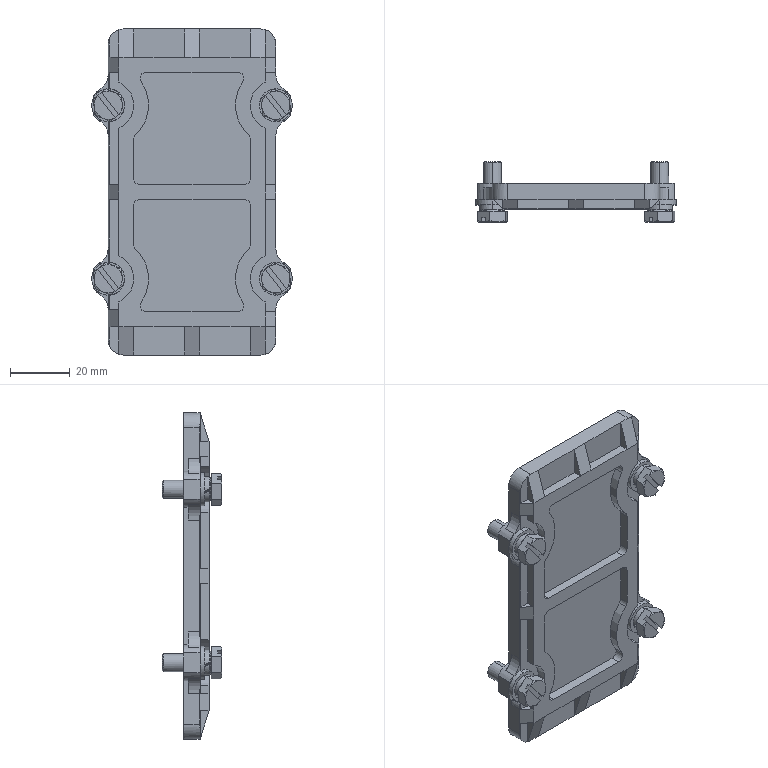Part | SolidWorks | features BaseBody 1 | 1 solid | 380 faces | box 67 x 20 x 109 mm | volume 32297 mm3 | plane 201 | cylinder 109 | cone 42 | spline 28 | commonest cylinder face diameters 6.5 x20 4 x12 8.5 x12 6 x8 6.4 x8 11 x8